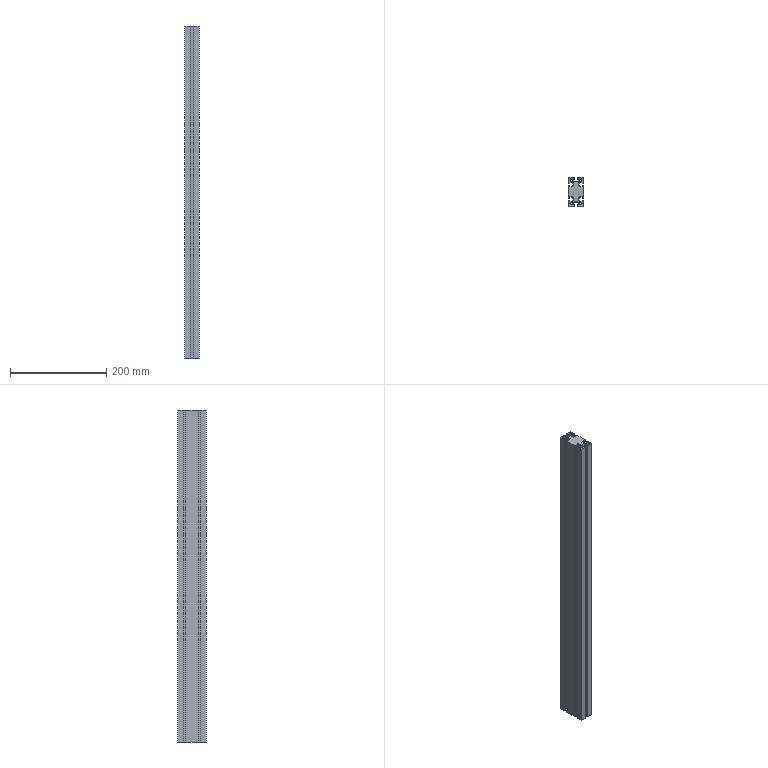Part | SolidWorks | features Extrusion 1 | 1 solid | 86 faces | box 30 x 60 x 690 mm | volume 830163 mm3 | plane 78 | cylinder 8 | commonest cylinder face diameters 6 x8